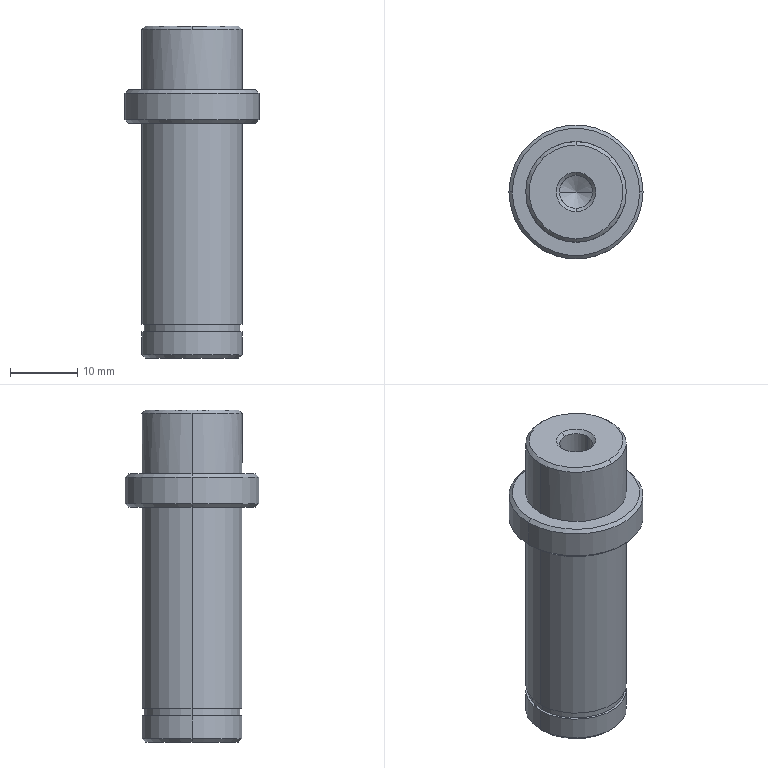Part | STEP file | Swing arm pivot shaft | 1 solid | 30 faces | box 20 x 20 x 49.5 mm | volume 9151 mm3 | cylinder 12 | cone 12 | plane 6 | commonest cylinder face diameters 15 x6 4.917 x2 14.3 x2 20 x2